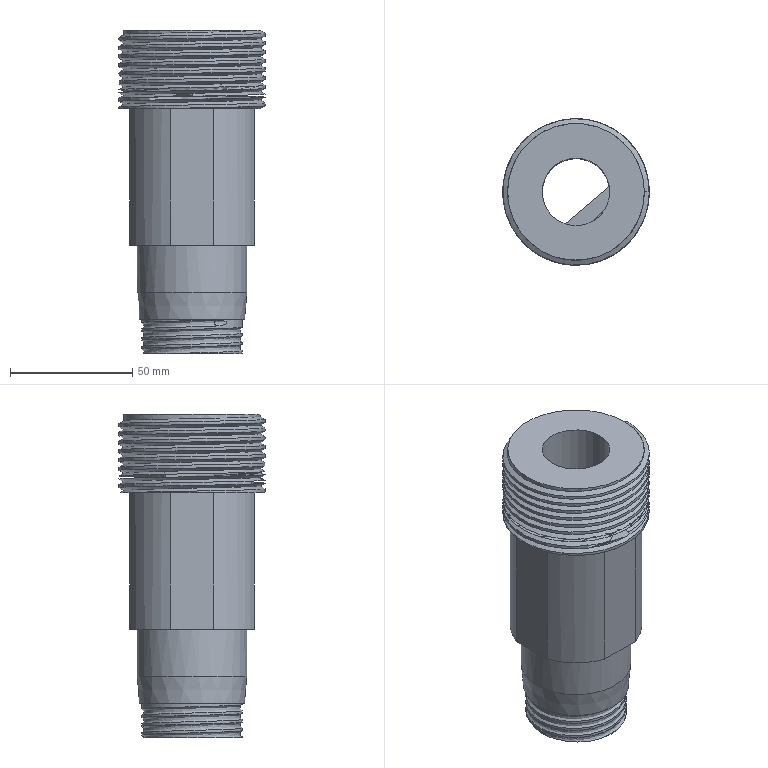Part | STEP file | SLIDE2-SCREW-AXS_id598_x_t | 1 solid | 43 faces | box 60.006 x 59.998 x 132.392 mm | volume 194092 mm3 | cylinder 14 | plane 13 | spline 12 | other 3 | cone 1 | commonest cylinder face diameters 41.229 x4 54 x4 27.69 x2 33.899 x1 34.917 x1 45 x1